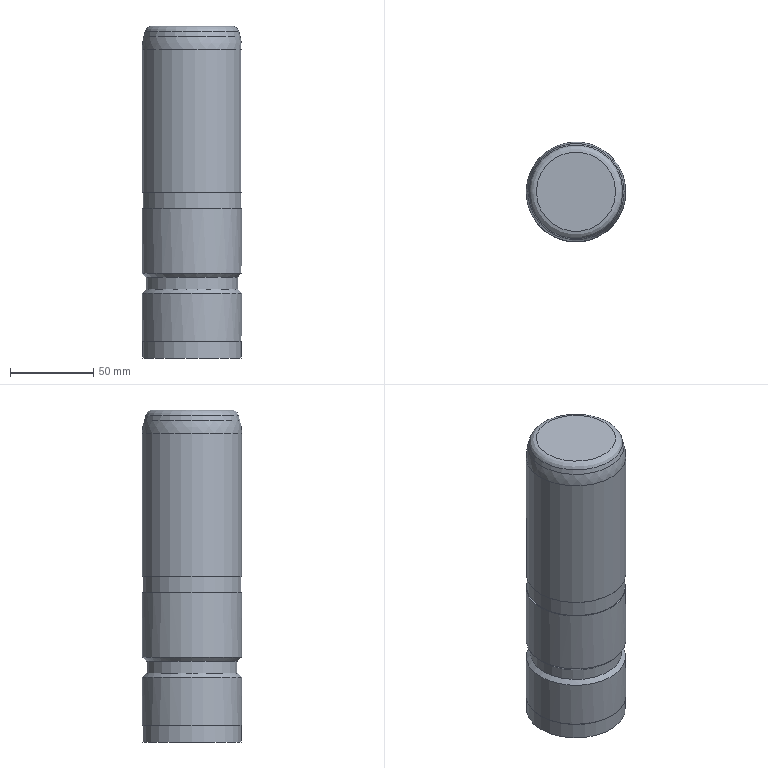Part | NX | features solid 2 | 1 solid | 16 faces | box 60 x 60 x 200 mm | volume 556815 mm3 | cylinder 6 | plane 5 | cone 3 | sphere 1 | torus 1 | commonest cylinder face diameters 60 x3 55 x1 59 x1 59.5 x1
STEP:
#1=CARTESIAN_POINT('',(827.5,175.,-101.5));
#2=VERTEX_POINT('',#1);
#3=CARTESIAN_POINT('',(800.,175.,-101.5));
#4=DIRECTION('',(0.,0.,1.));
#5=DIRECTION('',(1.,0.,0.));
#6=AXIS2_PLACEMENT_3D('',#3,#4,#5);
#7=CIRCLE('',#6,27.5);
#8=EDGE_CURVE('',#2,#2,#7,.T.);
#9=ORIENTED_EDGE('',*,*,#8,.T.);
#10=EDGE_LOOP('',(#9));
#11=FACE_BOUND('',#10,.T.);
#12=CARTESIAN_POINT('',(770.,175.,-99.));
#13=VERTEX_POINT('',#12);
#14=CARTESIAN_POINT('',(800.,175.,-99.));
#15=DIRECTION('',(0.,0.,-1.));
#16=DIRECTION('',(-1.,0.,0.));
#17=AXIS2_PLACEMENT_3D('',#14,#15,#16);
#18=CIRCLE('',#17,30.);
#19=EDGE_CURVE('',#13,#13,#18,.T.);
#20=ORIENTED_EDGE('',*,*,#19,.T.);
#21=EDGE_LOOP('',(#20));
#22=FACE_BOUND('',#21,.T.);
#23=CARTESIAN_POINT('',(800.,175.,-101.5));
#24=DIRECTION('',(0.,0.,1.));
#25=DIRECTION('',(-1.,0.,0.));
#26=AXIS2_PLACEMENT_3D('',#23,#24,#25);
#27=CONICAL_SURFACE('',#26,27.5,0.7854);
#28=ADVANCED_FACE('',(#11,#22),#27,.T.);
#29=ORIENTED_EDGE('',*,*,#8,.F.);
#30=EDGE_LOOP('',(#29));
#31=FACE_BOUND('',#30,.T.);
#32=CARTESIAN_POINT('',(827.5,175.,-108.5));
#33=VERTEX_POINT('',#32);
#34=CARTESIAN_POINT('',(800.,175.,-108.5));
#35=DIRECTION('',(0.,0.,1.));
#36=DIRECTION('',(1.,0.,0.));
#37=AXIS2_PLACEMENT_3D('',#34,#35,#36);
#38=CIRCLE('',#37,27.5);
#39=EDGE_CURVE('',#33,#33,#38,.T.);
#40=ORIENTED_EDGE('',*,*,#39,.T.);
#41=EDGE_LOOP('',(#40));
#42=FACE_BOUND('',#41,.T.);
#43=CARTESIAN_POINT('',(800.,175.,-108.5));
#44=DIRECTION('',(0.,0.,1.));
#45=DIRECTION('',(-1.,0.,0.));
#46=AXIS2_PLACEMENT_3D('',#43,#44,#45);
#47=CYLINDRICAL_SURFACE('',#46,27.5);
#48=ADVANCED_FACE('',(#31,#42),#47,.T.);
#49=CARTESIAN_POINT('',(770.5,175.,-60.));
#50=VERTEX_POINT('',#49);
#51=CARTESIAN_POINT('',(800.,175.,-60.));
#52=DIRECTION('',(0.,0.,-1.));
#53=DIRECTION('',(-1.,0.,0.));
#54=AXIS2_PLACEMENT_3D('',#51,#52,#53);
#55=CIRCLE('',#54,29.5);
#56=EDGE_CURVE('',#50,#50,#55,.T.);
#57=ORIENTED_EDGE('',*,*,#56,.T.);
#58=EDGE_LOOP('',(#57));
#59=FACE_BOUND('',#58,.T.);
#60=CARTESIAN_POINT('',(830.,175.,-60.));
#61=VERTEX_POINT('',#60);
#62=CARTESIAN_POINT('',(800.,175.,-60.));
#63=DIRECTION('',(0.,0.,1.));
#64=DIRECTION('',(1.,0.,0.));
#65=AXIS2_PLACEMENT_3D('',#62,#63,#64);
#66=CIRCLE('',#65,30.);
#67=EDGE_CURVE('',#61,#61,#66,.T.);
#68=ORIENTED_EDGE('',*,*,#67,.T.);
#69=EDGE_LOOP('',(#68));
#70=FACE_BOUND('',#69,.T.);
#71=CARTESIAN_POINT('',(800.,175.,-60.));
#72=DIRECTION('',(0.,0.,1.));
#73=DIRECTION('',(-1.,0.,0.));
#74=AXIS2_PLACEMENT_3D('',#71,#72,#73);
#75=PLANE('',#74);
#76=ADVANCED_FACE('',(#59,#70),#75,.T.);
#77=ORIENTED_EDGE('',*,*,#67,.F.);
#78=EDGE_LOOP('',(#77));
#79=FACE_BOUND('',#78,.T.);
#80=ORIENTED_EDGE('',*,*,#19,.F.);
#81=EDGE_LOOP('',(#80));
#82=FACE_BOUND('',#81,.T.);
#83=CARTESIAN_POINT('',(800.,175.,-99.));
#84=DIRECTION('',(0.,0.,1.));
#85=DIRECTION('',(-1.,0.,0.));
#86=AXIS2_PLACEMENT_3D('',#83,#84,#85);
#87=CYLINDRICAL_SURFACE('',#86,30.);
#88=ADVANCED_FACE('',(#79,#82),#87,.T.);
#89=CARTESIAN_POINT('',(829.5,175.,-50.));
#90=VERTEX_POINT('',#89);
#91=CARTESIAN_POINT('',(800.,175.,-50.));
#92=DIRECTION('',(0.,0.,1.));
#93=DIRECTION('',(1.,0.,0.));
#94=AXIS2_PLACEMENT_3D('',#91,#92,#93);
#95=CIRCLE('',#94,29.5);
#96=EDGE_CURVE('',#90,#90,#95,.T.);
#97=ORIENTED_EDGE('',*,*,#96,.T.);
#98=EDGE_LOOP('',(#97));
#99=FACE_BOUND('',#98,.T.);
#100=CARTESIAN_POINT('',(770.,175.,-50.));
#101=VERTEX_POINT('',#100);
#102=CARTESIAN_POINT('',(800.,175.,-50.));
#103=DIRECTION('',(0.,0.,-1.));
#104=DIRECTION('',(-1.,0.,0.));
#105=AXIS2_PLACEMENT_3D('',#102,#103,#104);
#106=CIRCLE('',#105,30.);
#107=EDGE_CURVE('',#101,#101,#106,.T.);
#108=ORIENTED_EDGE('',*,*,#107,.T.);
#109=EDGE_LOOP('',(#108));
#110=FACE_BOUND('',#109,.T.);
#111=CARTESIAN_POINT('',(800.,175.,-50.));
#112=DIRECTION('',(0.,0.,-1.));
#113=DIRECTION('',(1.,0.,0.));
#114=AXIS2_PLACEMENT_3D('',#111,#112,#113);
#115=PLANE('',#114);
#116=ADVANCED_FACE('',(#99,#110),#115,.T.);
#117=CARTESIAN_POINT('',(770.,175.,36.05));
#118=VERTEX_POINT('',#117);
#119=CARTESIAN_POINT('',(800.,175.,36.05));
#120=DIRECTION('',(0.,0.,-1.));
#121=DIRECTION('',(-1.,0.,0.));
#122=AXIS2_PLACEMENT_3D('',#119,#120,#121);
#123=CIRCLE('',#122,30.);
#124=EDGE_CURVE('',#118,#118,#123,.F.);
#125=ORIENTED_EDGE('',*,*,#124,.F.);
#126=EDGE_LOOP('',(#125));
#127=FACE_BOUND('',#126,.T.);
#128=ORIENTED_EDGE('',*,*,#107,.F.);
#129=EDGE_LOOP('',(#128));
#130=FACE_BOUND('',#129,.T.);
#131=CARTESIAN_POINT('',(800.,175.,-50.));
#132=DIRECTION('',(0.,0.,1.));
#133=DIRECTION('',(-1.,0.,0.));
#134=AXIS2_PLACEMENT_3D('',#131,#132,#133);
#135=CYLINDRICAL_SURFACE('',#134,30.);
#136=ADVANCED_FACE('',(#127,#130),#135,.T.);
#137=ORIENTED_EDGE('',*,*,#96,.F.);
#138=EDGE_LOOP('',(#137));
#139=FACE_BOUND('',#138,.T.);
#140=ORIENTED_EDGE('',*,*,#56,.F.);
#141=EDGE_LOOP('',(#140));
#142=FACE_BOUND('',#141,.T.);
#143=CARTESIAN_POINT('',(800.,175.,-60.));
#144=DIRECTION('',(0.,0.,1.));
#145=DIRECTION('',(-1.,0.,0.));
#146=AXIS2_PLACEMENT_3D('',#143,#144,#145);
#147=CYLINDRICAL_SURFACE('',#146,29.5);
#148=ADVANCED_FACE('',(#139,#142),#147,.T.);
#149=CARTESIAN_POINT('',(776.132,175.,50.));
#150=VERTEX_POINT('',#149);
#151=CARTESIAN_POINT('',(800.,175.,50.));
#152=DIRECTION('',(0.,0.,-1.));
#153=DIRECTION('',(-1.,0.,0.));
#154=AXIS2_PLACEMENT_3D('',#151,#152,#153);
#155=CIRCLE('',#154,23.868);
#156=EDGE_CURVE('',#150,#150,#155,.T.);
#157=ORIENTED_EDGE('',*,*,#156,.F.);
#158=EDGE_LOOP('',(#157));
#159=FACE_BOUND('',#158,.T.);
#160=CARTESIAN_POINT('',(800.,175.,50.));
#161=DIRECTION('',(0.,0.,1.));
#162=DIRECTION('',(-1.,0.,0.));
#163=AXIS2_PLACEMENT_3D('',#160,#161,#162);
#164=PLANE('',#163);
#165=ADVANCED_FACE('',(#159),#164,.T.);
#166=CARTESIAN_POINT('',(771.786,175.,46.665));
#167=VERTEX_POINT('',#166);
#168=CARTESIAN_POINT('',(800.,175.,46.665));
#169=DIRECTION('',(0.,0.,-1.));
#170=DIRECTION('',(-1.,0.,0.));
#171=AXIS2_PLACEMENT_3D('',#168,#169,#170);
#172=CIRCLE('',#171,28.214);
#173=EDGE_CURVE('',#167,#167,#172,.F.);
#174=ORIENTED_EDGE('',*,*,#173,.F.);
#175=EDGE_LOOP('',(#174));
#176=FACE_BOUND('',#175,.T.);
#177=CARTESIAN_POINT('',(828.978,175.,43.815));
#178=VERTEX_POINT('',#177);
#179=CARTESIAN_POINT('',(800.,175.,43.815));
#180=DIRECTION('',(0.,0.,1.));
#181=DIRECTION('',(1.,0.,0.));
#182=AXIS2_PLACEMENT_3D('',#179,#180,#181);
#183=CIRCLE('',#182,28.978);
#184=EDGE_CURVE('',#178,#178,#183,.F.);
#185=ORIENTED_EDGE('',*,*,#184,.F.);
#186=EDGE_LOOP('',(#185));
#187=FACE_BOUND('',#186,.T.);
#188=CARTESIAN_POINT('',(800.,175.,50.));
#189=DIRECTION('',(0.,0.,-1.));
#190=DIRECTION('',(1.,0.,0.));
#191=AXIS2_PLACEMENT_3D('',#188,#189,#190);
#192=CONICAL_SURFACE('',#191,27.32,0.2618);
#193=ADVANCED_FACE('',(#176,#187),#192,.T.);
#194=CARTESIAN_POINT('',(829.75,175.,-140.));
#195=VERTEX_POINT('',#194);
#196=CARTESIAN_POINT('',(800.,175.,-140.));
#197=DIRECTION('',(0.,0.,1.));
#198=DIRECTION('',(1.,0.,0.));
#199=AXIS2_PLACEMENT_3D('',#196,#197,#198);
#200=CIRCLE('',#199,29.75);
#201=EDGE_CURVE('',#195,#195,#200,.T.);
#202=ORIENTED_EDGE('',*,*,#201,.T.);
#203=EDGE_LOOP('',(#202));
#204=FACE_BOUND('',#203,.T.);
#205=CARTESIAN_POINT('',(770.,175.,-140.));
#206=VERTEX_POINT('',#205);
#207=CARTESIAN_POINT('',(800.,175.,-140.));
#208=DIRECTION('',(0.,0.,-1.));
#209=DIRECTION('',(-1.,0.,0.));
#210=AXIS2_PLACEMENT_3D('',#207,#208,#209);
#211=CIRCLE('',#210,30.);
#212=EDGE_CURVE('',#206,#206,#211,.T.);
#213=ORIENTED_EDGE('',*,*,#212,.T.);
#214=EDGE_LOOP('',(#213));
#215=FACE_BOUND('',#214,.T.);
#216=CARTESIAN_POINT('',(800.,175.,-140.));
#217=DIRECTION('',(0.,0.,-1.));
#218=DIRECTION('',(1.,0.,0.));
#219=AXIS2_PLACEMENT_3D('',#216,#217,#218);
#220=PLANE('',#219);
#221=ADVANCED_FACE('',(#204,#215),#220,.T.);
#222=CARTESIAN_POINT('',(770.,175.,-111.));
#223=VERTEX_POINT('',#222);
#224=CARTESIAN_POINT('',(800.,175.,-111.));
#225=DIRECTION('',(0.,0.,-1.));
#226=DIRECTION('',(-1.,0.,0.));
#227=AXIS2_PLACEMENT_3D('',#224,#225,#226);
#228=CIRCLE('',#227,30.);
#229=EDGE_CURVE('',#223,#223,#228,.T.);
#230=ORIENTED_EDGE('',*,*,#229,.T.);
#231=EDGE_LOOP('',(#230));
#232=FACE_BOUND('',#231,.T.);
#233=ORIENTED_EDGE('',*,*,#212,.F.);
#234=EDGE_LOOP('',(#233));
#235=FACE_BOUND('',#234,.T.);
#236=CARTESIAN_POINT('',(800.,175.,-140.));
#237=DIRECTION('',(0.,0.,1.));
#238=DIRECTION('',(-1.,0.,0.));
#239=AXIS2_PLACEMENT_3D('',#236,#237,#238);
#240=CYLINDRICAL_SURFACE('',#239,30.);
#241=ADVANCED_FACE('',(#232,#235),#240,.T.);
#242=CARTESIAN_POINT('',(770.25,175.,-150.));
#243=VERTEX_POINT('',#242);
#244=CARTESIAN_POINT('',(800.,175.,-150.));
#245=DIRECTION('',(0.,0.,-1.));
#246=DIRECTION('',(-1.,0.,0.));
#247=AXIS2_PLACEMENT_3D('',#244,#245,#246);
#248=CIRCLE('',#247,29.75);
#249=EDGE_CURVE('',#243,#243,#248,.T.);
#250=ORIENTED_EDGE('',*,*,#249,.T.);
#251=EDGE_LOOP('',(#250));
#252=FACE_BOUND('',#251,.T.);
#253=CARTESIAN_POINT('',(800.,175.,-150.));
#254=DIRECTION('',(0.,0.,-1.));
#255=DIRECTION('',(1.,0.,0.));
#256=AXIS2_PLACEMENT_3D('',#253,#254,#255);
#257=PLANE('',#256);
#258=ADVANCED_FACE('',(#252),#257,.T.);
#259=ORIENTED_EDGE('',*,*,#201,.F.);
#260=EDGE_LOOP('',(#259));
#261=FACE_BOUND('',#260,.T.);
#262=ORIENTED_EDGE('',*,*,#249,.F.);
#263=EDGE_LOOP('',(#262));
#264=FACE_BOUND('',#263,.T.);
#265=CARTESIAN_POINT('',(800.,175.,-150.));
#266=DIRECTION('',(0.,0.,1.));
#267=DIRECTION('',(-1.,0.,0.));
#268=AXIS2_PLACEMENT_3D('',#265,#266,#267);
#269=CYLINDRICAL_SURFACE('',#268,29.75);
#270=ADVANCED_FACE('',(#261,#264),#269,.T.);
#271=ORIENTED_EDGE('',*,*,#229,.F.);
#272=EDGE_LOOP('',(#271));
#273=FACE_BOUND('',#272,.T.);
#274=ORIENTED_EDGE('',*,*,#39,.F.);
#275=EDGE_LOOP('',(#274));
#276=FACE_BOUND('',#275,.T.);
#277=CARTESIAN_POINT('',(800.,175.,-108.5));
#278=DIRECTION('',(0.,0.,-1.));
#279=DIRECTION('',(1.,0.,0.));
#280=AXIS2_PLACEMENT_3D('',#277,#278,#279);
#281=CONICAL_SURFACE('',#280,27.5,0.7854);
#282=ADVANCED_FACE('',(#273,#276),#281,.T.);
#283=ORIENTED_EDGE('',*,*,#124,.T.);
#284=EDGE_LOOP('',(#283));
#285=FACE_BOUND('',#284,.T.);
#286=ORIENTED_EDGE('',*,*,#184,.T.);
#287=EDGE_LOOP('',(#286));
#288=FACE_BOUND('',#287,.T.);
#289=CARTESIAN_POINT('',(800.,175.,36.05));
#290=DIRECTION('',(0.,0.,1.));
#291=DIRECTION('',(-1.,0.,0.));
#292=AXIS2_PLACEMENT_3D('',#289,#290,#291);
#293=SPHERICAL_SURFACE('',#292,30.);
#294=ADVANCED_FACE('',(#285,#288),#293,.T.);
#295=ORIENTED_EDGE('',*,*,#156,.T.);
#296=EDGE_LOOP('',(#295));
#297=FACE_BOUND('',#296,.T.);
#298=ORIENTED_EDGE('',*,*,#173,.T.);
#299=EDGE_LOOP('',(#298));
#300=FACE_BOUND('',#299,.T.);
#301=CARTESIAN_POINT('',(800.,175.,45.5));
#302=DIRECTION('',(0.,0.,1.));
#303=DIRECTION('',(-1.,0.,0.));
#304=AXIS2_PLACEMENT_3D('',#301,#302,#303);
#305=TOROIDAL_SURFACE('',#304,23.868,4.5);
#306=ADVANCED_FACE('',(#297,#300),#305,.T.);
#307=CLOSED_SHELL('',(#28,#48,#76,#88,#116,#136,#148,#165,#193,#221,#241,#258,#270,#282,#294,#306));
#308=MANIFOLD_SOLID_BREP('',#307);
#309=(LENGTH_UNIT()NAMED_UNIT(*)SI_UNIT(.MILLI.,.METRE.));
#310=UNCERTAINTY_MEASURE_WITH_UNIT(LENGTH_MEASURE(0.00001),#309,'','');
#311=(NAMED_UNIT(*)PLANE_ANGLE_UNIT()SI_UNIT($,.RADIAN.));
#312=(NAMED_UNIT(*)SI_UNIT($,.STERADIAN.)SOLID_ANGLE_UNIT());
#313=(GEOMETRIC_REPRESENTATION_CONTEXT(3)GLOBAL_UNCERTAINTY_ASSIGNED_CONTEXT((#310))GLOBAL_UNIT_ASSIGNED_CONTEXT((#309,#311,#312))REPRESENTATION_CONTEXT('',''));
#314=ADVANCED_BREP_SHAPE_REPRESENTATION('',(#308),#313);